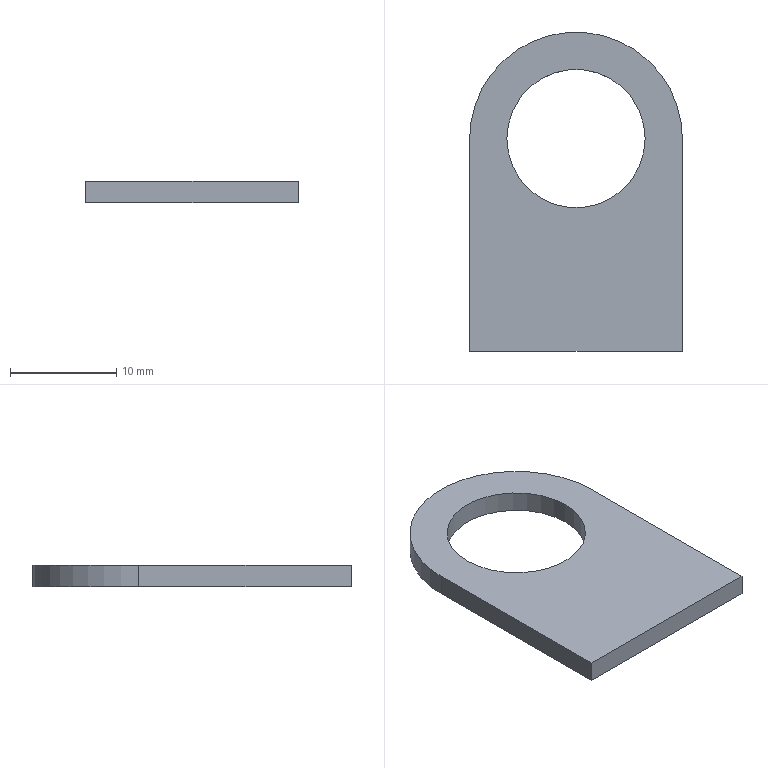Part | STEP file | PN_0014_default | 1 solid | 7 faces | box 20 x 30 x 2 mm | volume 848.625 mm3 | plane 5 | cylinder 2 | commonest cylinder face diameters 13 x1 20 x1
STEP:
#1=CARTESIAN_POINT('',(0.,0.,0.));
#2=DIRECTION('',(0.,0.,1.));
#3=DIRECTION('',(1.,0.,0.));
#4=AXIS2_PLACEMENT_3D('',#1,#2,#3);
#5=CARTESIAN_POINT('',(6.5,20.,1.));
#6=VERTEX_POINT('',#5);
#7=CARTESIAN_POINT('',(0.,20.,1.));
#8=DIRECTION('',(0.,0.,1.));
#9=DIRECTION('',(1.,0.,0.));
#10=AXIS2_PLACEMENT_3D('',#7,#8,#9);
#11=CIRCLE('',#10,6.5);
#12=CARTESIAN_POINT('',(0.,20.,1.));
#13=DIRECTION('',(0.,0.,-1.));
#14=DIRECTION('',(-1.,0.,0.));
#15=AXIS2_PLACEMENT_3D('',#12,#13,#14);
#16=PLANE('',#15);
#17=CARTESIAN_POINT('',(-6.5,0.));
#18=CARTESIAN_POINT('',(-6.5,11.258));
#19=CARTESIAN_POINT('',(3.25,5.629));
#20=CARTESIAN_POINT('',(13.,0.));
#21=CARTESIAN_POINT('',(3.25,-5.629));
#22=CARTESIAN_POINT('',(-6.5,-11.258));
#23=CARTESIAN_POINT('',(-6.5,0.));
#24=(BOUNDED_CURVE()B_SPLINE_CURVE(2,(#17,#18,#19,#20,#21,#22,#23),.UNSPECIFIED.,.T.,.F.)B_SPLINE_CURVE_WITH_KNOTS((1,2,2,2,2,1),(-2.094,0.,2.094,4.189,6.283,8.378),.UNSPECIFIED.)CURVE()GEOMETRIC_REPRESENTATION_ITEM()RATIONAL_B_SPLINE_CURVE((1.,0.5,1.,0.5,1.,0.5,1.))REPRESENTATION_ITEM(''));
#25=(GEOMETRIC_REPRESENTATION_CONTEXT(2)PARAMETRIC_REPRESENTATION_CONTEXT()REPRESENTATION_CONTEXT('',''));
#26=DEFINITIONAL_REPRESENTATION('',(#24),#25);
#27=PCURVE('',#16,#26);
#28=CARTESIAN_POINT('',(0.,20.,1.));
#29=DIRECTION('',(0.,0.,-1.));
#30=DIRECTION('',(-1.,0.,0.));
#31=AXIS2_PLACEMENT_3D('',#28,#29,#30);
#32=CYLINDRICAL_SURFACE('',#31,6.5);
#33=CARTESIAN_POINT('',(9.425,0.));
#34=DIRECTION('',(-1.,0.));
#35=VECTOR('',#34,1.);
#36=LINE('',#33,#35);
#37=(GEOMETRIC_REPRESENTATION_CONTEXT(2)PARAMETRIC_REPRESENTATION_CONTEXT()REPRESENTATION_CONTEXT('',''));
#38=DEFINITIONAL_REPRESENTATION('',(#36),#37);
#39=PCURVE('',#32,#38);
#40=SURFACE_CURVE('',#11,(#27,#39),.PCURVE_S1.);
#41=EDGE_CURVE('',#6,#6,#40,.T.);
#42=ORIENTED_EDGE('',*,*,#41,.F.);
#43=EDGE_LOOP('',(#42));
#44=FACE_BOUND('',#43,.T.);
#45=CARTESIAN_POINT('',(10.,0.,1.));
#46=VERTEX_POINT('',#45);
#47=CARTESIAN_POINT('',(-10.,0.003491,1.));
#48=VERTEX_POINT('',#47);
#49=CARTESIAN_POINT('',(-0.00349,0.001746,1.));
#50=DIRECTION('',(-1.,0.0001745,0.));
#51=VECTOR('',#50,1.);
#52=LINE('',#49,#51);
#53=CARTESIAN_POINT('',(0.00349,-19.998));
#54=DIRECTION('',(1.,0.0001745));
#55=VECTOR('',#54,1.);
#56=LINE('',#53,#55);
#57=(GEOMETRIC_REPRESENTATION_CONTEXT(2)PARAMETRIC_REPRESENTATION_CONTEXT()REPRESENTATION_CONTEXT('',''));
#58=DEFINITIONAL_REPRESENTATION('',(#56),#57);
#59=PCURVE('',#16,#58);
#60=CARTESIAN_POINT('',(10.,0.,46.139));
#61=DIRECTION('',(-0.0001745,-1.,0.));
#62=DIRECTION('',(1.,-0.0001745,0.));
#63=AXIS2_PLACEMENT_3D('',#60,#61,#62);
#64=PLANE('',#63);
#65=CARTESIAN_POINT('',(-10.003,-45.139));
#66=DIRECTION('',(-1.,0.));
#67=VECTOR('',#66,1.);
#68=LINE('',#65,#67);
#69=(GEOMETRIC_REPRESENTATION_CONTEXT(2)PARAMETRIC_REPRESENTATION_CONTEXT()REPRESENTATION_CONTEXT('',''));
#70=DEFINITIONAL_REPRESENTATION('',(#68),#69);
#71=PCURVE('',#64,#70);
#72=SURFACE_CURVE('',#52,(#59,#71),.PCURVE_S1.);
#73=EDGE_CURVE('',#46,#48,#72,.T.);
#74=ORIENTED_EDGE('',*,*,#73,.F.);
#75=CARTESIAN_POINT('',(10.,20.,1.));
#76=VERTEX_POINT('',#75);
#77=CARTESIAN_POINT('',(10.,0.,1.));
#78=DIRECTION('',(0.,1.,0.));
#79=VECTOR('',#78,1.);
#80=LINE('',#77,#79);
#81=CARTESIAN_POINT('',(-10.,-20.));
#82=DIRECTION('',(0.,1.));
#83=VECTOR('',#82,1.);
#84=LINE('',#81,#83);
#85=(GEOMETRIC_REPRESENTATION_CONTEXT(2)PARAMETRIC_REPRESENTATION_CONTEXT()REPRESENTATION_CONTEXT('',''));
#86=DEFINITIONAL_REPRESENTATION('',(#84),#85);
#87=PCURVE('',#16,#86);
#88=CARTESIAN_POINT('',(10.,0.,1.));
#89=DIRECTION('',(-1.,0.,0.));
#90=DIRECTION('',(0.,-1.,0.));
#91=AXIS2_PLACEMENT_3D('',#88,#89,#90);
#92=PLANE('',#91);
#93=CARTESIAN_POINT('',(0.,0.));
#94=DIRECTION('',(-1.,0.));
#95=VECTOR('',#94,1.);
#96=LINE('',#93,#95);
#97=(GEOMETRIC_REPRESENTATION_CONTEXT(2)PARAMETRIC_REPRESENTATION_CONTEXT()REPRESENTATION_CONTEXT('',''));
#98=DEFINITIONAL_REPRESENTATION('',(#96),#97);
#99=PCURVE('',#92,#98);
#100=SURFACE_CURVE('',#80,(#87,#99),.PCURVE_S1.);
#101=EDGE_CURVE('',#46,#76,#100,.T.);
#102=ORIENTED_EDGE('',*,*,#101,.T.);
#103=CARTESIAN_POINT('',(-10.,20.,1.));
#104=VERTEX_POINT('',#103);
#105=CARTESIAN_POINT('',(0.,20.,1.));
#106=DIRECTION('',(0.,0.,1.));
#107=DIRECTION('',(-1.,0.,0.));
#108=AXIS2_PLACEMENT_3D('',#105,#106,#107);
#109=CIRCLE('',#108,10.);
#110=CARTESIAN_POINT('',(10.,0.));
#111=CARTESIAN_POINT('',(10.,-17.321));
#112=CARTESIAN_POINT('',(-5.,-8.66));
#113=CARTESIAN_POINT('',(-20.,0.));
#114=CARTESIAN_POINT('',(-5.,8.66));
#115=CARTESIAN_POINT('',(10.,17.321));
#116=CARTESIAN_POINT('',(10.,0.));
#117=(BOUNDED_CURVE()B_SPLINE_CURVE(2,(#110,#111,#112,#113,#114,#115,#116),.UNSPECIFIED.,.T.,.F.)B_SPLINE_CURVE_WITH_KNOTS((1,2,2,2,2,1),(-2.094,0.,2.094,4.189,6.283,8.378),.UNSPECIFIED.)CURVE()GEOMETRIC_REPRESENTATION_ITEM()RATIONAL_B_SPLINE_CURVE((1.,0.5,1.,0.5,1.,0.5,1.))REPRESENTATION_ITEM(''));
#118=(GEOMETRIC_REPRESENTATION_CONTEXT(2)PARAMETRIC_REPRESENTATION_CONTEXT()REPRESENTATION_CONTEXT('',''));
#119=DEFINITIONAL_REPRESENTATION('',(#117),#118);
#120=PCURVE('',#16,#119);
#121=CARTESIAN_POINT('',(0.,20.,1.));
#122=DIRECTION('',(0.,0.,-1.));
#123=DIRECTION('',(-1.,0.,0.));
#124=AXIS2_PLACEMENT_3D('',#121,#122,#123);
#125=CYLINDRICAL_SURFACE('',#124,10.);
#126=CARTESIAN_POINT('',(6.283,0.));
#127=DIRECTION('',(-1.,0.));
#128=VECTOR('',#127,1.);
#129=LINE('',#126,#128);
#130=(GEOMETRIC_REPRESENTATION_CONTEXT(2)PARAMETRIC_REPRESENTATION_CONTEXT()REPRESENTATION_CONTEXT('',''));
#131=DEFINITIONAL_REPRESENTATION('',(#129),#130);
#132=PCURVE('',#125,#131);
#133=SURFACE_CURVE('',#109,(#120,#132),.PCURVE_S1.);
#134=EDGE_CURVE('',#76,#104,#133,.T.);
#135=ORIENTED_EDGE('',*,*,#134,.T.);
#136=CARTESIAN_POINT('',(-10.,0.,1.));
#137=DIRECTION('',(0.,-1.,0.));
#138=VECTOR('',#137,1.);
#139=LINE('',#136,#138);
#140=CARTESIAN_POINT('',(10.,-20.));
#141=DIRECTION('',(0.,-1.));
#142=VECTOR('',#141,1.);
#143=LINE('',#140,#142);
#144=(GEOMETRIC_REPRESENTATION_CONTEXT(2)PARAMETRIC_REPRESENTATION_CONTEXT()REPRESENTATION_CONTEXT('',''));
#145=DEFINITIONAL_REPRESENTATION('',(#143),#144);
#146=PCURVE('',#16,#145);
#147=CARTESIAN_POINT('',(-10.,0.,1.));
#148=DIRECTION('',(1.,0.,0.));
#149=DIRECTION('',(0.,1.,0.));
#150=AXIS2_PLACEMENT_3D('',#147,#148,#149);
#151=PLANE('',#150);
#152=CARTESIAN_POINT('',(0.,0.));
#153=DIRECTION('',(-1.,0.));
#154=VECTOR('',#153,1.);
#155=LINE('',#152,#154);
#156=(GEOMETRIC_REPRESENTATION_CONTEXT(2)PARAMETRIC_REPRESENTATION_CONTEXT()REPRESENTATION_CONTEXT('',''));
#157=DEFINITIONAL_REPRESENTATION('',(#155),#156);
#158=PCURVE('',#151,#157);
#159=SURFACE_CURVE('',#139,(#146,#158),.PCURVE_S1.);
#160=EDGE_CURVE('',#104,#48,#159,.T.);
#161=ORIENTED_EDGE('',*,*,#160,.T.);
#162=EDGE_LOOP('',(#74,#102,#135,#161));
#163=FACE_BOUND('',#162,.T.);
#164=ADVANCED_FACE('',(#44,#163),#16,.F.);
#165=CARTESIAN_POINT('',(6.5,20.,-1.));
#166=VERTEX_POINT('',#165);
#167=CARTESIAN_POINT('',(0.,20.,-1.));
#168=DIRECTION('',(0.,0.,1.));
#169=DIRECTION('',(1.,0.,0.));
#170=AXIS2_PLACEMENT_3D('',#167,#168,#169);
#171=CIRCLE('',#170,6.5);
#172=CARTESIAN_POINT('',(0.,20.,-1.));
#173=DIRECTION('',(0.,0.,-1.));
#174=DIRECTION('',(-1.,0.,0.));
#175=AXIS2_PLACEMENT_3D('',#172,#173,#174);
#176=PLANE('',#175);
#177=CARTESIAN_POINT('',(-6.5,0.));
#178=CARTESIAN_POINT('',(-6.5,11.258));
#179=CARTESIAN_POINT('',(3.25,5.629));
#180=CARTESIAN_POINT('',(13.,0.));
#181=CARTESIAN_POINT('',(3.25,-5.629));
#182=CARTESIAN_POINT('',(-6.5,-11.258));
#183=CARTESIAN_POINT('',(-6.5,0.));
#184=(BOUNDED_CURVE()B_SPLINE_CURVE(2,(#177,#178,#179,#180,#181,#182,#183),.UNSPECIFIED.,.T.,.F.)B_SPLINE_CURVE_WITH_KNOTS((1,2,2,2,2,1),(-2.094,0.,2.094,4.189,6.283,8.378),.UNSPECIFIED.)CURVE()GEOMETRIC_REPRESENTATION_ITEM()RATIONAL_B_SPLINE_CURVE((1.,0.5,1.,0.5,1.,0.5,1.))REPRESENTATION_ITEM(''));
#185=(GEOMETRIC_REPRESENTATION_CONTEXT(2)PARAMETRIC_REPRESENTATION_CONTEXT()REPRESENTATION_CONTEXT('',''));
#186=DEFINITIONAL_REPRESENTATION('',(#184),#185);
#187=PCURVE('',#176,#186);
#188=CARTESIAN_POINT('',(9.425,2.));
#189=DIRECTION('',(-1.,0.));
#190=VECTOR('',#189,1.);
#191=LINE('',#188,#190);
#192=(GEOMETRIC_REPRESENTATION_CONTEXT(2)PARAMETRIC_REPRESENTATION_CONTEXT()REPRESENTATION_CONTEXT('',''));
#193=DEFINITIONAL_REPRESENTATION('',(#191),#192);
#194=PCURVE('',#32,#193);
#195=SURFACE_CURVE('',#171,(#187,#194),.PCURVE_S1.);
#196=EDGE_CURVE('',#166,#166,#195,.T.);
#197=ORIENTED_EDGE('',*,*,#196,.T.);
#198=EDGE_LOOP('',(#197));
#199=FACE_BOUND('',#198,.T.);
#200=CARTESIAN_POINT('',(10.,0.,-1.));
#201=VERTEX_POINT('',#200);
#202=CARTESIAN_POINT('',(10.,20.,-1.));
#203=VERTEX_POINT('',#202);
#204=CARTESIAN_POINT('',(10.,0.,-1.));
#205=DIRECTION('',(0.,1.,0.));
#206=VECTOR('',#205,1.);
#207=LINE('',#204,#206);
#208=CARTESIAN_POINT('',(-10.,-20.));
#209=DIRECTION('',(0.,1.));
#210=VECTOR('',#209,1.);
#211=LINE('',#208,#210);
#212=(GEOMETRIC_REPRESENTATION_CONTEXT(2)PARAMETRIC_REPRESENTATION_CONTEXT()REPRESENTATION_CONTEXT('',''));
#213=DEFINITIONAL_REPRESENTATION('',(#211),#212);
#214=PCURVE('',#176,#213);
#215=CARTESIAN_POINT('',(0.,-2.));
#216=DIRECTION('',(-1.,0.));
#217=VECTOR('',#216,1.);
#218=LINE('',#215,#217);
#219=(GEOMETRIC_REPRESENTATION_CONTEXT(2)PARAMETRIC_REPRESENTATION_CONTEXT()REPRESENTATION_CONTEXT('',''));
#220=DEFINITIONAL_REPRESENTATION('',(#218),#219);
#221=PCURVE('',#92,#220);
#222=SURFACE_CURVE('',#207,(#214,#221),.PCURVE_S1.);
#223=EDGE_CURVE('',#201,#203,#222,.T.);
#224=ORIENTED_EDGE('',*,*,#223,.F.);
#225=CARTESIAN_POINT('',(-10.,0.003491,-1.));
#226=VERTEX_POINT('',#225);
#227=CARTESIAN_POINT('',(-0.00349,0.001746,-1.));
#228=DIRECTION('',(-1.,0.0001745,0.));
#229=VECTOR('',#228,1.);
#230=LINE('',#227,#229);
#231=CARTESIAN_POINT('',(0.00349,-19.998));
#232=DIRECTION('',(1.,0.0001745));
#233=VECTOR('',#232,1.);
#234=LINE('',#231,#233);
#235=(GEOMETRIC_REPRESENTATION_CONTEXT(2)PARAMETRIC_REPRESENTATION_CONTEXT()REPRESENTATION_CONTEXT('',''));
#236=DEFINITIONAL_REPRESENTATION('',(#234),#235);
#237=PCURVE('',#176,#236);
#238=CARTESIAN_POINT('',(-10.003,-47.139));
#239=DIRECTION('',(-1.,0.));
#240=VECTOR('',#239,1.);
#241=LINE('',#238,#240);
#242=(GEOMETRIC_REPRESENTATION_CONTEXT(2)PARAMETRIC_REPRESENTATION_CONTEXT()REPRESENTATION_CONTEXT('',''));
#243=DEFINITIONAL_REPRESENTATION('',(#241),#242);
#244=PCURVE('',#64,#243);
#245=SURFACE_CURVE('',#230,(#237,#244),.PCURVE_S1.);
#246=EDGE_CURVE('',#201,#226,#245,.T.);
#247=ORIENTED_EDGE('',*,*,#246,.T.);
#248=CARTESIAN_POINT('',(-10.,20.,-1.));
#249=VERTEX_POINT('',#248);
#250=CARTESIAN_POINT('',(-10.,0.,-1.));
#251=DIRECTION('',(0.,-1.,0.));
#252=VECTOR('',#251,1.);
#253=LINE('',#250,#252);
#254=CARTESIAN_POINT('',(10.,-20.));
#255=DIRECTION('',(0.,-1.));
#256=VECTOR('',#255,1.);
#257=LINE('',#254,#256);
#258=(GEOMETRIC_REPRESENTATION_CONTEXT(2)PARAMETRIC_REPRESENTATION_CONTEXT()REPRESENTATION_CONTEXT('',''));
#259=DEFINITIONAL_REPRESENTATION('',(#257),#258);
#260=PCURVE('',#176,#259);
#261=CARTESIAN_POINT('',(0.,-2.));
#262=DIRECTION('',(-1.,0.));
#263=VECTOR('',#262,1.);
#264=LINE('',#261,#263);
#265=(GEOMETRIC_REPRESENTATION_CONTEXT(2)PARAMETRIC_REPRESENTATION_CONTEXT()REPRESENTATION_CONTEXT('',''));
#266=DEFINITIONAL_REPRESENTATION('',(#264),#265);
#267=PCURVE('',#151,#266);
#268=SURFACE_CURVE('',#253,(#260,#267),.PCURVE_S1.);
#269=EDGE_CURVE('',#249,#226,#268,.T.);
#270=ORIENTED_EDGE('',*,*,#269,.F.);
#271=CARTESIAN_POINT('',(0.,20.,-1.));
#272=DIRECTION('',(0.,0.,1.));
#273=DIRECTION('',(-1.,0.,0.));
#274=AXIS2_PLACEMENT_3D('',#271,#272,#273);
#275=CIRCLE('',#274,10.);
#276=CARTESIAN_POINT('',(10.,0.));
#277=CARTESIAN_POINT('',(10.,-17.321));
#278=CARTESIAN_POINT('',(-5.,-8.66));
#279=CARTESIAN_POINT('',(-20.,0.));
#280=CARTESIAN_POINT('',(-5.,8.66));
#281=CARTESIAN_POINT('',(10.,17.321));
#282=CARTESIAN_POINT('',(10.,0.));
#283=(BOUNDED_CURVE()B_SPLINE_CURVE(2,(#276,#277,#278,#279,#280,#281,#282),.UNSPECIFIED.,.T.,.F.)B_SPLINE_CURVE_WITH_KNOTS((1,2,2,2,2,1),(-2.094,0.,2.094,4.189,6.283,8.378),.UNSPECIFIED.)CURVE()GEOMETRIC_REPRESENTATION_ITEM()RATIONAL_B_SPLINE_CURVE((1.,0.5,1.,0.5,1.,0.5,1.))REPRESENTATION_ITEM(''));
#284=(GEOMETRIC_REPRESENTATION_CONTEXT(2)PARAMETRIC_REPRESENTATION_CONTEXT()REPRESENTATION_CONTEXT('',''));
#285=DEFINITIONAL_REPRESENTATION('',(#283),#284);
#286=PCURVE('',#176,#285);
#287=CARTESIAN_POINT('',(6.283,2.));
#288=DIRECTION('',(-1.,0.));
#289=VECTOR('',#288,1.);
#290=LINE('',#287,#289);
#291=(GEOMETRIC_REPRESENTATION_CONTEXT(2)PARAMETRIC_REPRESENTATION_CONTEXT()REPRESENTATION_CONTEXT('',''));
#292=DEFINITIONAL_REPRESENTATION('',(#290),#291);
#293=PCURVE('',#125,#292);
#294=SURFACE_CURVE('',#275,(#286,#293),.PCURVE_S1.);
#295=EDGE_CURVE('',#203,#249,#294,.T.);
#296=ORIENTED_EDGE('',*,*,#295,.F.);
#297=EDGE_LOOP('',(#224,#247,#270,#296));
#298=FACE_BOUND('',#297,.T.);
#299=ADVANCED_FACE('',(#199,#298),#176,.T.);
#300=CARTESIAN_POINT('',(-10.,0.003491,1.));
#301=DIRECTION('',(0.,0.,-1.));
#302=VECTOR('',#301,1.);
#303=LINE('',#300,#302);
#304=CARTESIAN_POINT('',(0.003491,0.));
#305=DIRECTION('',(0.,-1.));
#306=VECTOR('',#305,1.);
#307=LINE('',#304,#306);
#308=(GEOMETRIC_REPRESENTATION_CONTEXT(2)PARAMETRIC_REPRESENTATION_CONTEXT()REPRESENTATION_CONTEXT('',''));
#309=DEFINITIONAL_REPRESENTATION('',(#307),#308);
#310=PCURVE('',#151,#309);
#311=CARTESIAN_POINT('',(-20.,-45.139));
#312=DIRECTION('',(0.,-1.));
#313=VECTOR('',#312,1.);
#314=LINE('',#311,#313);
#315=(GEOMETRIC_REPRESENTATION_CONTEXT(2)PARAMETRIC_REPRESENTATION_CONTEXT()REPRESENTATION_CONTEXT('',''));
#316=DEFINITIONAL_REPRESENTATION('',(#314),#315);
#317=PCURVE('',#64,#316);
#318=SURFACE_CURVE('',#303,(#310,#317),.PCURVE_S1.);
#319=EDGE_CURVE('',#48,#226,#318,.T.);
#320=ORIENTED_EDGE('',*,*,#319,.F.);
#321=ORIENTED_EDGE('',*,*,#160,.F.);
#322=CARTESIAN_POINT('',(-10.,20.,1.));
#323=DIRECTION('',(0.,0.,-1.));
#324=VECTOR('',#323,1.);
#325=LINE('',#322,#324);
#326=CARTESIAN_POINT('',(20.,0.));
#327=DIRECTION('',(0.,-1.));
#328=VECTOR('',#327,1.);
#329=LINE('',#326,#328);
#330=(GEOMETRIC_REPRESENTATION_CONTEXT(2)PARAMETRIC_REPRESENTATION_CONTEXT()REPRESENTATION_CONTEXT('',''));
#331=DEFINITIONAL_REPRESENTATION('',(#329),#330);
#332=PCURVE('',#151,#331);
#333=CARTESIAN_POINT('',(0.,0.));
#334=DIRECTION('',(0.,1.));
#335=VECTOR('',#334,1.);
#336=LINE('',#333,#335);
#337=(GEOMETRIC_REPRESENTATION_CONTEXT(2)PARAMETRIC_REPRESENTATION_CONTEXT()REPRESENTATION_CONTEXT('',''));
#338=DEFINITIONAL_REPRESENTATION('',(#336),#337);
#339=PCURVE('',#125,#338);
#340=SURFACE_CURVE('',#325,(#332,#339),.PCURVE_S1.);
#341=EDGE_CURVE('',#104,#249,#340,.T.);
#342=ORIENTED_EDGE('',*,*,#341,.T.);
#343=ORIENTED_EDGE('',*,*,#269,.T.);
#344=EDGE_LOOP('',(#320,#321,#342,#343));
#345=FACE_BOUND('',#344,.T.);
#346=ADVANCED_FACE('',(#345),#151,.F.);
#347=ORIENTED_EDGE('',*,*,#223,.T.);
#348=CARTESIAN_POINT('',(10.,20.,1.));
#349=DIRECTION('',(0.,0.,-1.));
#350=VECTOR('',#349,1.);
#351=LINE('',#348,#350);
#352=CARTESIAN_POINT('',(-20.,0.));
#353=DIRECTION('',(0.,-1.));
#354=VECTOR('',#353,1.);
#355=LINE('',#352,#354);
#356=(GEOMETRIC_REPRESENTATION_CONTEXT(2)PARAMETRIC_REPRESENTATION_CONTEXT()REPRESENTATION_CONTEXT('',''));
#357=DEFINITIONAL_REPRESENTATION('',(#355),#356);
#358=PCURVE('',#92,#357);
#359=CARTESIAN_POINT('',(3.142,0.));
#360=DIRECTION('',(0.,1.));
#361=VECTOR('',#360,1.);
#362=LINE('',#359,#361);
#363=(GEOMETRIC_REPRESENTATION_CONTEXT(2)PARAMETRIC_REPRESENTATION_CONTEXT()REPRESENTATION_CONTEXT('',''));
#364=DEFINITIONAL_REPRESENTATION('',(#362),#363);
#365=PCURVE('',#125,#364);
#366=SURFACE_CURVE('',#351,(#358,#365),.PCURVE_S1.);
#367=EDGE_CURVE('',#76,#203,#366,.T.);
#368=ORIENTED_EDGE('',*,*,#367,.F.);
#369=ORIENTED_EDGE('',*,*,#101,.F.);
#370=CARTESIAN_POINT('',(10.,0.,1.));
#371=DIRECTION('',(0.,0.,-1.));
#372=VECTOR('',#371,1.);
#373=LINE('',#370,#372);
#374=CARTESIAN_POINT('',(0.,0.));
#375=DIRECTION('',(0.,-1.));
#376=VECTOR('',#375,1.);
#377=LINE('',#374,#376);
#378=(GEOMETRIC_REPRESENTATION_CONTEXT(2)PARAMETRIC_REPRESENTATION_CONTEXT()REPRESENTATION_CONTEXT('',''));
#379=DEFINITIONAL_REPRESENTATION('',(#377),#378);
#380=PCURVE('',#92,#379);
#381=CARTESIAN_POINT('',(0.,-45.139));
#382=DIRECTION('',(0.,-1.));
#383=VECTOR('',#382,1.);
#384=LINE('',#381,#383);
#385=(GEOMETRIC_REPRESENTATION_CONTEXT(2)PARAMETRIC_REPRESENTATION_CONTEXT()REPRESENTATION_CONTEXT('',''));
#386=DEFINITIONAL_REPRESENTATION('',(#384),#385);
#387=PCURVE('',#64,#386);
#388=SURFACE_CURVE('',#373,(#380,#387),.PCURVE_S1.);
#389=EDGE_CURVE('',#46,#201,#388,.T.);
#390=ORIENTED_EDGE('',*,*,#389,.T.);
#391=EDGE_LOOP('',(#347,#368,#369,#390));
#392=FACE_BOUND('',#391,.T.);
#393=ADVANCED_FACE('',(#392),#92,.F.);
#394=ORIENTED_EDGE('',*,*,#295,.T.);
#395=ORIENTED_EDGE('',*,*,#341,.F.);
#396=ORIENTED_EDGE('',*,*,#134,.F.);
#397=ORIENTED_EDGE('',*,*,#367,.T.);
#398=EDGE_LOOP('',(#394,#395,#396,#397));
#399=FACE_BOUND('',#398,.T.);
#400=ADVANCED_FACE('',(#399),#125,.T.);
#401=ORIENTED_EDGE('',*,*,#41,.F.);
#402=CARTESIAN_POINT('',(6.5,20.,1.));
#403=CARTESIAN_POINT('',(6.5,20.,-1.));
#404=B_SPLINE_CURVE_WITH_KNOTS('',1,(#402,#403),.UNSPECIFIED.,.F.,.F.,(2,2),(0.,2.),.PIECEWISE_BEZIER_KNOTS.);
#405=CARTESIAN_POINT('',(9.425,0.));
#406=DIRECTION('',(0.,1.));
#407=VECTOR('',#406,1.);
#408=LINE('',#405,#407);
#409=(GEOMETRIC_REPRESENTATION_CONTEXT(2)PARAMETRIC_REPRESENTATION_CONTEXT()REPRESENTATION_CONTEXT('',''));
#410=DEFINITIONAL_REPRESENTATION('',(#408),#409);
#411=PCURVE('',#32,#410);
#412=CARTESIAN_POINT('',(3.142,0.));
#413=DIRECTION('',(0.,1.));
#414=VECTOR('',#413,1.);
#415=LINE('',#412,#414);
#416=(GEOMETRIC_REPRESENTATION_CONTEXT(2)PARAMETRIC_REPRESENTATION_CONTEXT()REPRESENTATION_CONTEXT('',''));
#417=DEFINITIONAL_REPRESENTATION('',(#415),#416);
#418=PCURVE('',#32,#417);
#419=SEAM_CURVE('',#404,(#411,#418),.PCURVE_S1.);
#420=EDGE_CURVE('',#6,#166,#419,.T.);
#421=ORIENTED_EDGE('',*,*,#420,.T.);
#422=ORIENTED_EDGE('',*,*,#196,.T.);
#423=ORIENTED_EDGE('',*,*,#420,.F.);
#424=EDGE_LOOP('',(#401,#421,#422,#423));
#425=FACE_BOUND('',#424,.F.);
#426=ADVANCED_FACE('',(#425),#32,.F.);
#427=ORIENTED_EDGE('',*,*,#389,.F.);
#428=ORIENTED_EDGE('',*,*,#73,.T.);
#429=ORIENTED_EDGE('',*,*,#319,.T.);
#430=ORIENTED_EDGE('',*,*,#246,.F.);
#431=EDGE_LOOP('',(#427,#428,#429,#430));
#432=FACE_BOUND('',#431,.T.);
#433=ADVANCED_FACE('',(#432),#64,.T.);
#434=CLOSED_SHELL('',(#164,#299,#346,#393,#400,#426,#433));
#435=MANIFOLD_SOLID_BREP('',#434);
#436=(LENGTH_UNIT()NAMED_UNIT(*)SI_UNIT(.MILLI.,.METRE.));
#437=UNCERTAINTY_MEASURE_WITH_UNIT(LENGTH_MEASURE(0.000002),#436,'','');
#438=(NAMED_UNIT(*)PLANE_ANGLE_UNIT()SI_UNIT($,.RADIAN.));
#439=(NAMED_UNIT(*)SI_UNIT($,.STERADIAN.)SOLID_ANGLE_UNIT());
#440=(GEOMETRIC_REPRESENTATION_CONTEXT(3)GLOBAL_UNCERTAINTY_ASSIGNED_CONTEXT((#437))GLOBAL_UNIT_ASSIGNED_CONTEXT((#436,#438,#439))REPRESENTATION_CONTEXT('',''));
#441=ADVANCED_BREP_SHAPE_REPRESENTATION('',(#4,#435),#440);